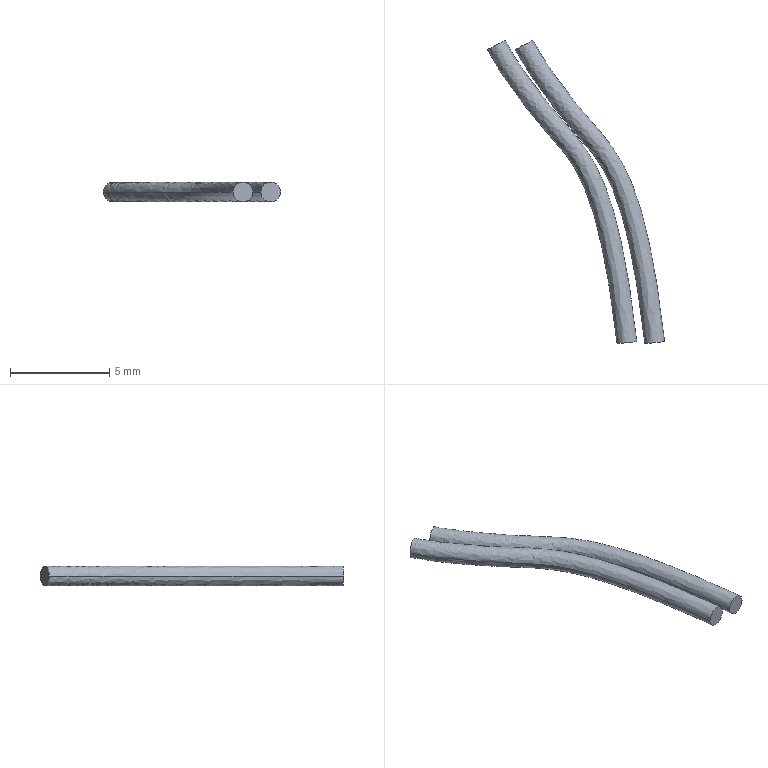Part | SolidWorks | features BaseBody 2 | 2 solids | 8 faces | box 8.921 x 15.285 x 1 mm | volume 26.359 mm3 | plane 4 | spline 4
STEP:
#1=CARTESIAN_POINT('',(-0.4968,-0.05673,0.));
#2=VERTEX_POINT('',#1);
#3=CARTESIAN_POINT('',(0.4968,0.05673,0.));
#4=VERTEX_POINT('',#3);
#5=CARTESIAN_POINT('',(0.,0.,0.));
#6=DIRECTION('',(-0.1135,0.9935,0.));
#7=DIRECTION('',(-0.9935,-0.1135,0.));
#8=AXIS2_PLACEMENT_3D('',#5,#6,#7);
#9=CIRCLE('',#8,0.5);
#10=EDGE_CURVE('',#2,#4,#9,.T.);
#11=ORIENTED_EDGE('',*,*,#10,.F.);
#12=CARTESIAN_POINT('',(0.,0.,0.));
#13=DIRECTION('',(-0.1135,0.9935,0.));
#14=DIRECTION('',(-0.9935,-0.1135,0.));
#15=AXIS2_PLACEMENT_3D('',#12,#13,#14);
#16=CIRCLE('',#15,0.5);
#17=EDGE_CURVE('',#4,#2,#16,.T.);
#18=ORIENTED_EDGE('',*,*,#17,.F.);
#19=EDGE_LOOP('',(#11,#18));
#20=FACE_OUTER_BOUND('',#19,.T.);
#21=CARTESIAN_POINT('',(0.,0.,0.));
#22=DIRECTION('',(-0.1135,0.9935,0.));
#23=DIRECTION('',(0.,0.,1.));
#24=AXIS2_PLACEMENT_3D('',#21,#22,#23);
#25=PLANE('',#24);
#26=ADVANCED_FACE('',(#20),#25,.F.);
#27=CARTESIAN_POINT('',(-7.024,14.772,0.));
#28=VERTEX_POINT('',#27);
#29=CARTESIAN_POINT('',(-6.134,15.228,0.));
#30=VERTEX_POINT('',#29);
#31=CARTESIAN_POINT('',(-6.579,15.,0.));
#32=DIRECTION('',(-0.4556,0.8902,0.));
#33=DIRECTION('',(-0.8902,-0.4556,0.));
#34=AXIS2_PLACEMENT_3D('',#31,#32,#33);
#35=CIRCLE('',#34,0.5);
#36=EDGE_CURVE('',#28,#30,#35,.T.);
#37=ORIENTED_EDGE('',*,*,#36,.T.);
#38=CARTESIAN_POINT('',(-6.579,15.,0.));
#39=DIRECTION('',(-0.4556,0.8902,0.));
#40=DIRECTION('',(-0.8902,-0.4556,0.));
#41=AXIS2_PLACEMENT_3D('',#38,#39,#40);
#42=CIRCLE('',#41,0.5);
#43=EDGE_CURVE('',#30,#28,#42,.T.);
#44=ORIENTED_EDGE('',*,*,#43,.T.);
#45=EDGE_LOOP('',(#37,#44));
#46=FACE_OUTER_BOUND('',#45,.T.);
#47=CARTESIAN_POINT('',(-6.579,15.,0.));
#48=DIRECTION('',(-0.4556,0.8902,0.));
#49=DIRECTION('',(0.,0.,1.));
#50=AXIS2_PLACEMENT_3D('',#47,#48,#49);
#51=PLANE('',#50);
#52=ADVANCED_FACE('',(#46),#51,.T.);
#53=CARTESIAN_POINT('',(0.4968,0.05673,0.));
#54=CARTESIAN_POINT('',(0.03588,4.093,0.));
#55=CARTESIAN_POINT('',(-0.5239,6.452,0.));
#56=CARTESIAN_POINT('',(-1.773,9.573,0.));
#57=CARTESIAN_POINT('',(-2.484,10.33,0.));
#58=CARTESIAN_POINT('',(-4.339,12.439,0.));
#59=CARTESIAN_POINT('',(-5.518,14.024,0.));
#60=CARTESIAN_POINT('',(-6.134,15.228,0.));
#61=B_SPLINE_CURVE_WITH_KNOTS('',3,(#53,#54,#55,#56,#57,#58,#59,#60),.UNSPECIFIED.,.F.,.F.,(4,2,2,4),(0.,0.2491,0.4982,1.),.UNSPECIFIED.);
#62=EDGE_CURVE('',#4,#30,#61,.T.);
#63=ORIENTED_EDGE('',*,*,#62,.F.);
#64=ORIENTED_EDGE('',*,*,#17,.T.);
#65=CARTESIAN_POINT('',(-0.4968,-0.05673,0.));
#66=CARTESIAN_POINT('',(-0.9522,3.932,0.));
#67=CARTESIAN_POINT('',(-1.505,6.213,0.));
#68=CARTESIAN_POINT('',(-2.648,9.069,0.));
#69=CARTESIAN_POINT('',(-3.217,9.649,0.));
#70=CARTESIAN_POINT('',(-5.126,11.82,0.));
#71=CARTESIAN_POINT('',(-6.337,13.429,0.));
#72=CARTESIAN_POINT('',(-7.024,14.772,0.));
#73=B_SPLINE_CURVE_WITH_KNOTS('',3,(#65,#66,#67,#68,#69,#70,#71,#72),.UNSPECIFIED.,.F.,.F.,(4,2,2,4),(0.,0.2491,0.4982,1.),.UNSPECIFIED.);
#74=EDGE_CURVE('',#2,#28,#73,.T.);
#75=ORIENTED_EDGE('',*,*,#74,.T.);
#76=ORIENTED_EDGE('',*,*,#43,.F.);
#77=EDGE_LOOP('',(#63,#64,#75,#76));
#78=FACE_OUTER_BOUND('',#77,.T.);
#79=CARTESIAN_POINT('',(0.4968,0.05673,0.));
#80=CARTESIAN_POINT('',(0.03588,4.093,0.));
#81=CARTESIAN_POINT('',(-0.5239,6.452,0.));
#82=CARTESIAN_POINT('',(-1.773,9.573,0.));
#83=CARTESIAN_POINT('',(-2.484,10.33,0.));
#84=CARTESIAN_POINT('',(-4.339,12.439,0.));
#85=CARTESIAN_POINT('',(-5.518,14.024,0.));
#86=CARTESIAN_POINT('',(-6.134,15.228,0.));
#87=CARTESIAN_POINT('',(0.4968,0.05673,-1.));
#88=CARTESIAN_POINT('',(0.03588,4.093,-1.));
#89=CARTESIAN_POINT('',(-0.5239,6.452,-1.));
#90=CARTESIAN_POINT('',(-1.773,9.573,-1.));
#91=CARTESIAN_POINT('',(-2.484,10.33,-1.));
#92=CARTESIAN_POINT('',(-4.339,12.439,-1.));
#93=CARTESIAN_POINT('',(-5.518,14.024,-1.));
#94=CARTESIAN_POINT('',(-6.134,15.228,-1.));
#95=CARTESIAN_POINT('',(-0.4968,-0.05673,-1.));
#96=CARTESIAN_POINT('',(-0.9522,3.932,-1.));
#97=CARTESIAN_POINT('',(-1.505,6.213,-1.));
#98=CARTESIAN_POINT('',(-2.648,9.069,-1.));
#99=CARTESIAN_POINT('',(-3.217,9.649,-1.));
#100=CARTESIAN_POINT('',(-5.126,11.82,-1.));
#101=CARTESIAN_POINT('',(-6.337,13.429,-1.));
#102=CARTESIAN_POINT('',(-7.024,14.772,-1.));
#103=CARTESIAN_POINT('',(-0.4968,-0.05673,0.));
#104=CARTESIAN_POINT('',(-0.9522,3.932,0.));
#105=CARTESIAN_POINT('',(-1.505,6.213,0.));
#106=CARTESIAN_POINT('',(-2.648,9.069,0.));
#107=CARTESIAN_POINT('',(-3.217,9.649,0.));
#108=CARTESIAN_POINT('',(-5.126,11.82,0.));
#109=CARTESIAN_POINT('',(-6.337,13.429,0.));
#110=CARTESIAN_POINT('',(-7.024,14.772,0.));
#111=(BOUNDED_SURFACE()B_SPLINE_SURFACE(3,3,((#79,#80,#81,#82,#83,#84,#85,#86),(#87,#88,#89,#90,#91,#92,#93,#94),(#95,#96,#97,#98,#99,#100,#101,#102),(#103,#104,#105,#106,#107,#108,#109,#110)),.UNSPECIFIED.,.F.,.F.,.F.)B_SPLINE_SURFACE_WITH_KNOTS((4,4),(4,2,2,4),(0.5,1.),(0.,0.2491,0.4982,1.),.UNSPECIFIED.)GEOMETRIC_REPRESENTATION_ITEM()RATIONAL_B_SPLINE_SURFACE(((1.,1.,1.,1.,1.,1.,1.,1.),(0.3333,0.3333,0.3333,0.3333,0.3333,0.3333,0.3333,0.3333),(0.3333,0.3333,0.3333,0.3333,0.3333,0.3333,0.3333,0.3333),(1.,1.,1.,1.,1.,1.,1.,1.)))REPRESENTATION_ITEM('')SURFACE());
#112=ADVANCED_FACE('',(#78),#111,.T.);
#113=ORIENTED_EDGE('',*,*,#10,.T.);
#114=ORIENTED_EDGE('',*,*,#62,.T.);
#115=ORIENTED_EDGE('',*,*,#36,.F.);
#116=ORIENTED_EDGE('',*,*,#74,.F.);
#117=EDGE_LOOP('',(#113,#114,#115,#116));
#118=FACE_OUTER_BOUND('',#117,.T.);
#119=CARTESIAN_POINT('',(-0.4968,-0.05673,0.));
#120=CARTESIAN_POINT('',(-0.9522,3.932,0.));
#121=CARTESIAN_POINT('',(-1.505,6.213,0.));
#122=CARTESIAN_POINT('',(-2.648,9.069,0.));
#123=CARTESIAN_POINT('',(-3.217,9.649,0.));
#124=CARTESIAN_POINT('',(-5.126,11.82,0.));
#125=CARTESIAN_POINT('',(-6.337,13.429,0.));
#126=CARTESIAN_POINT('',(-7.024,14.772,0.));
#127=CARTESIAN_POINT('',(-0.4968,-0.05673,1.));
#128=CARTESIAN_POINT('',(-0.9522,3.932,1.));
#129=CARTESIAN_POINT('',(-1.505,6.213,1.));
#130=CARTESIAN_POINT('',(-2.648,9.069,1.));
#131=CARTESIAN_POINT('',(-3.217,9.649,1.));
#132=CARTESIAN_POINT('',(-5.126,11.82,1.));
#133=CARTESIAN_POINT('',(-6.337,13.429,1.));
#134=CARTESIAN_POINT('',(-7.024,14.772,1.));
#135=CARTESIAN_POINT('',(0.4968,0.05673,1.));
#136=CARTESIAN_POINT('',(0.03588,4.093,1.));
#137=CARTESIAN_POINT('',(-0.5239,6.452,1.));
#138=CARTESIAN_POINT('',(-1.773,9.573,1.));
#139=CARTESIAN_POINT('',(-2.484,10.33,1.));
#140=CARTESIAN_POINT('',(-4.339,12.439,1.));
#141=CARTESIAN_POINT('',(-5.518,14.024,1.));
#142=CARTESIAN_POINT('',(-6.134,15.228,1.));
#143=CARTESIAN_POINT('',(0.4968,0.05673,0.));
#144=CARTESIAN_POINT('',(0.03588,4.093,0.));
#145=CARTESIAN_POINT('',(-0.5239,6.452,0.));
#146=CARTESIAN_POINT('',(-1.773,9.573,0.));
#147=CARTESIAN_POINT('',(-2.484,10.33,0.));
#148=CARTESIAN_POINT('',(-4.339,12.439,0.));
#149=CARTESIAN_POINT('',(-5.518,14.024,0.));
#150=CARTESIAN_POINT('',(-6.134,15.228,0.));
#151=(BOUNDED_SURFACE()B_SPLINE_SURFACE(3,3,((#119,#120,#121,#122,#123,#124,#125,#126),(#127,#128,#129,#130,#131,#132,#133,#134),(#135,#136,#137,#138,#139,#140,#141,#142),(#143,#144,#145,#146,#147,#148,#149,#150)),.UNSPECIFIED.,.F.,.F.,.F.)B_SPLINE_SURFACE_WITH_KNOTS((4,4),(4,2,2,4),(0.,0.5),(0.,0.2491,0.4982,1.),.UNSPECIFIED.)GEOMETRIC_REPRESENTATION_ITEM()RATIONAL_B_SPLINE_SURFACE(((1.,1.,1.,1.,1.,1.,1.,1.),(0.3333,0.3333,0.3333,0.3333,0.3333,0.3333,0.3333,0.3333),(0.3333,0.3333,0.3333,0.3333,0.3333,0.3333,0.3333,0.3333),(1.,1.,1.,1.,1.,1.,1.,1.)))REPRESENTATION_ITEM('')SURFACE());
#152=ADVANCED_FACE('',(#118),#151,.T.);
#153=CLOSED_SHELL('',(#26,#52,#112,#152));
#154=MANIFOLD_SOLID_BREP('',#153);
#155=CARTESIAN_POINT('',(0.9032,-0.05673,0.));
#156=VERTEX_POINT('',#155);
#157=CARTESIAN_POINT('',(1.897,0.05673,0.));
#158=VERTEX_POINT('',#157);
#159=CARTESIAN_POINT('',(1.4,0.,0.));
#160=DIRECTION('',(-0.1135,0.9935,0.));
#161=DIRECTION('',(-0.9935,-0.1135,0.));
#162=AXIS2_PLACEMENT_3D('',#159,#160,#161);
#163=CIRCLE('',#162,0.5);
#164=EDGE_CURVE('',#156,#158,#163,.T.);
#165=ORIENTED_EDGE('',*,*,#164,.F.);
#166=CARTESIAN_POINT('',(1.4,0.,0.));
#167=DIRECTION('',(-0.1135,0.9935,0.));
#168=DIRECTION('',(-0.9935,-0.1135,0.));
#169=AXIS2_PLACEMENT_3D('',#166,#167,#168);
#170=CIRCLE('',#169,0.5);
#171=EDGE_CURVE('',#158,#156,#170,.T.);
#172=ORIENTED_EDGE('',*,*,#171,.F.);
#173=EDGE_LOOP('',(#165,#172));
#174=FACE_OUTER_BOUND('',#173,.T.);
#175=CARTESIAN_POINT('',(1.4,0.,0.));
#176=DIRECTION('',(-0.1135,0.9935,0.));
#177=DIRECTION('',(0.,0.,1.));
#178=AXIS2_PLACEMENT_3D('',#175,#176,#177);
#179=PLANE('',#178);
#180=ADVANCED_FACE('',(#174),#179,.F.);
#181=CARTESIAN_POINT('',(-5.624,14.772,0.));
#182=VERTEX_POINT('',#181);
#183=CARTESIAN_POINT('',(-4.734,15.228,0.));
#184=VERTEX_POINT('',#183);
#185=CARTESIAN_POINT('',(-5.179,15.,0.));
#186=DIRECTION('',(-0.4556,0.8902,0.));
#187=DIRECTION('',(-0.8902,-0.4556,0.));
#188=AXIS2_PLACEMENT_3D('',#185,#186,#187);
#189=CIRCLE('',#188,0.5);
#190=EDGE_CURVE('',#182,#184,#189,.T.);
#191=ORIENTED_EDGE('',*,*,#190,.T.);
#192=CARTESIAN_POINT('',(-5.179,15.,0.));
#193=DIRECTION('',(-0.4556,0.8902,0.));
#194=DIRECTION('',(-0.8902,-0.4556,0.));
#195=AXIS2_PLACEMENT_3D('',#192,#193,#194);
#196=CIRCLE('',#195,0.5);
#197=EDGE_CURVE('',#184,#182,#196,.T.);
#198=ORIENTED_EDGE('',*,*,#197,.T.);
#199=EDGE_LOOP('',(#191,#198));
#200=FACE_OUTER_BOUND('',#199,.T.);
#201=CARTESIAN_POINT('',(-5.179,15.,0.));
#202=DIRECTION('',(-0.4556,0.8902,0.));
#203=DIRECTION('',(0.,0.,1.));
#204=AXIS2_PLACEMENT_3D('',#201,#202,#203);
#205=PLANE('',#204);
#206=ADVANCED_FACE('',(#200),#205,.T.);
#207=CARTESIAN_POINT('',(1.897,0.05673,0.));
#208=CARTESIAN_POINT('',(1.436,4.093,0.));
#209=CARTESIAN_POINT('',(0.8761,6.452,0.));
#210=CARTESIAN_POINT('',(-0.3732,9.573,0.));
#211=CARTESIAN_POINT('',(-1.084,10.33,0.));
#212=CARTESIAN_POINT('',(-2.939,12.439,0.));
#213=CARTESIAN_POINT('',(-4.118,14.024,0.));
#214=CARTESIAN_POINT('',(-4.734,15.228,0.));
#215=B_SPLINE_CURVE_WITH_KNOTS('',3,(#207,#208,#209,#210,#211,#212,#213,#214),.UNSPECIFIED.,.F.,.F.,(4,2,2,4),(0.,0.2491,0.4982,1.),.UNSPECIFIED.);
#216=EDGE_CURVE('',#158,#184,#215,.T.);
#217=ORIENTED_EDGE('',*,*,#216,.F.);
#218=ORIENTED_EDGE('',*,*,#171,.T.);
#219=CARTESIAN_POINT('',(0.9032,-0.05673,0.));
#220=CARTESIAN_POINT('',(0.4478,3.932,0.));
#221=CARTESIAN_POINT('',(-0.1055,6.213,0.));
#222=CARTESIAN_POINT('',(-1.248,9.069,0.));
#223=CARTESIAN_POINT('',(-1.817,9.649,0.));
#224=CARTESIAN_POINT('',(-3.726,11.82,0.));
#225=CARTESIAN_POINT('',(-4.937,13.429,0.));
#226=CARTESIAN_POINT('',(-5.624,14.772,0.));
#227=B_SPLINE_CURVE_WITH_KNOTS('',3,(#219,#220,#221,#222,#223,#224,#225,#226),.UNSPECIFIED.,.F.,.F.,(4,2,2,4),(0.,0.2491,0.4982,1.),.UNSPECIFIED.);
#228=EDGE_CURVE('',#156,#182,#227,.T.);
#229=ORIENTED_EDGE('',*,*,#228,.T.);
#230=ORIENTED_EDGE('',*,*,#197,.F.);
#231=EDGE_LOOP('',(#217,#218,#229,#230));
#232=FACE_OUTER_BOUND('',#231,.T.);
#233=CARTESIAN_POINT('',(1.897,0.05673,0.));
#234=CARTESIAN_POINT('',(1.436,4.093,0.));
#235=CARTESIAN_POINT('',(0.8761,6.452,0.));
#236=CARTESIAN_POINT('',(-0.3732,9.573,0.));
#237=CARTESIAN_POINT('',(-1.084,10.33,0.));
#238=CARTESIAN_POINT('',(-2.939,12.439,0.));
#239=CARTESIAN_POINT('',(-4.118,14.024,0.));
#240=CARTESIAN_POINT('',(-4.734,15.228,0.));
#241=CARTESIAN_POINT('',(1.897,0.05673,-1.));
#242=CARTESIAN_POINT('',(1.436,4.093,-1.));
#243=CARTESIAN_POINT('',(0.8761,6.452,-1.));
#244=CARTESIAN_POINT('',(-0.3732,9.573,-1.));
#245=CARTESIAN_POINT('',(-1.084,10.33,-1.));
#246=CARTESIAN_POINT('',(-2.939,12.439,-1.));
#247=CARTESIAN_POINT('',(-4.118,14.024,-1.));
#248=CARTESIAN_POINT('',(-4.734,15.228,-1.));
#249=CARTESIAN_POINT('',(0.9032,-0.05673,-1.));
#250=CARTESIAN_POINT('',(0.4478,3.932,-1.));
#251=CARTESIAN_POINT('',(-0.1055,6.213,-1.));
#252=CARTESIAN_POINT('',(-1.248,9.069,-1.));
#253=CARTESIAN_POINT('',(-1.817,9.649,-1.));
#254=CARTESIAN_POINT('',(-3.726,11.82,-1.));
#255=CARTESIAN_POINT('',(-4.937,13.429,-1.));
#256=CARTESIAN_POINT('',(-5.624,14.772,-1.));
#257=CARTESIAN_POINT('',(0.9032,-0.05673,0.));
#258=CARTESIAN_POINT('',(0.4478,3.932,0.));
#259=CARTESIAN_POINT('',(-0.1055,6.213,0.));
#260=CARTESIAN_POINT('',(-1.248,9.069,0.));
#261=CARTESIAN_POINT('',(-1.817,9.649,0.));
#262=CARTESIAN_POINT('',(-3.726,11.82,0.));
#263=CARTESIAN_POINT('',(-4.937,13.429,0.));
#264=CARTESIAN_POINT('',(-5.624,14.772,0.));
#265=(BOUNDED_SURFACE()B_SPLINE_SURFACE(3,3,((#233,#234,#235,#236,#237,#238,#239,#240),(#241,#242,#243,#244,#245,#246,#247,#248),(#249,#250,#251,#252,#253,#254,#255,#256),(#257,#258,#259,#260,#261,#262,#263,#264)),.UNSPECIFIED.,.F.,.F.,.T.)B_SPLINE_SURFACE_WITH_KNOTS((4,4),(4,2,2,4),(0.5,1.),(0.,0.2491,0.4982,1.),.UNSPECIFIED.)GEOMETRIC_REPRESENTATION_ITEM()RATIONAL_B_SPLINE_SURFACE(((1.,1.,1.,1.,1.,1.,1.,1.),(0.3333,0.3333,0.3333,0.3333,0.3333,0.3333,0.3333,0.3333),(0.3333,0.3333,0.3333,0.3333,0.3333,0.3333,0.3333,0.3333),(1.,1.,1.,1.,1.,1.,1.,1.)))REPRESENTATION_ITEM('')SURFACE());
#266=ADVANCED_FACE('',(#232),#265,.T.);
#267=ORIENTED_EDGE('',*,*,#164,.T.);
#268=ORIENTED_EDGE('',*,*,#216,.T.);
#269=ORIENTED_EDGE('',*,*,#190,.F.);
#270=ORIENTED_EDGE('',*,*,#228,.F.);
#271=EDGE_LOOP('',(#267,#268,#269,#270));
#272=FACE_OUTER_BOUND('',#271,.T.);
#273=CARTESIAN_POINT('',(0.9032,-0.05673,0.));
#274=CARTESIAN_POINT('',(0.4478,3.932,0.));
#275=CARTESIAN_POINT('',(-0.1055,6.213,0.));
#276=CARTESIAN_POINT('',(-1.248,9.069,0.));
#277=CARTESIAN_POINT('',(-1.817,9.649,0.));
#278=CARTESIAN_POINT('',(-3.726,11.82,0.));
#279=CARTESIAN_POINT('',(-4.937,13.429,0.));
#280=CARTESIAN_POINT('',(-5.624,14.772,0.));
#281=CARTESIAN_POINT('',(0.9032,-0.05673,1.));
#282=CARTESIAN_POINT('',(0.4478,3.932,1.));
#283=CARTESIAN_POINT('',(-0.1055,6.213,1.));
#284=CARTESIAN_POINT('',(-1.248,9.069,1.));
#285=CARTESIAN_POINT('',(-1.817,9.649,1.));
#286=CARTESIAN_POINT('',(-3.726,11.82,1.));
#287=CARTESIAN_POINT('',(-4.937,13.429,1.));
#288=CARTESIAN_POINT('',(-5.624,14.772,1.));
#289=CARTESIAN_POINT('',(1.897,0.05673,1.));
#290=CARTESIAN_POINT('',(1.436,4.093,1.));
#291=CARTESIAN_POINT('',(0.8761,6.452,1.));
#292=CARTESIAN_POINT('',(-0.3732,9.573,1.));
#293=CARTESIAN_POINT('',(-1.084,10.33,1.));
#294=CARTESIAN_POINT('',(-2.939,12.439,1.));
#295=CARTESIAN_POINT('',(-4.118,14.024,1.));
#296=CARTESIAN_POINT('',(-4.734,15.228,1.));
#297=CARTESIAN_POINT('',(1.897,0.05673,0.));
#298=CARTESIAN_POINT('',(1.436,4.093,0.));
#299=CARTESIAN_POINT('',(0.8761,6.452,0.));
#300=CARTESIAN_POINT('',(-0.3732,9.573,0.));
#301=CARTESIAN_POINT('',(-1.084,10.33,0.));
#302=CARTESIAN_POINT('',(-2.939,12.439,0.));
#303=CARTESIAN_POINT('',(-4.118,14.024,0.));
#304=CARTESIAN_POINT('',(-4.734,15.228,0.));
#305=(BOUNDED_SURFACE()B_SPLINE_SURFACE(3,3,((#273,#274,#275,#276,#277,#278,#279,#280),(#281,#282,#283,#284,#285,#286,#287,#288),(#289,#290,#291,#292,#293,#294,#295,#296),(#297,#298,#299,#300,#301,#302,#303,#304)),.UNSPECIFIED.,.F.,.F.,.F.)B_SPLINE_SURFACE_WITH_KNOTS((4,4),(4,2,2,4),(0.,0.5),(0.,0.2491,0.4982,1.),.UNSPECIFIED.)GEOMETRIC_REPRESENTATION_ITEM()RATIONAL_B_SPLINE_SURFACE(((1.,1.,1.,1.,1.,1.,1.,1.),(0.3333,0.3333,0.3333,0.3333,0.3333,0.3333,0.3333,0.3333),(0.3333,0.3333,0.3333,0.3333,0.3333,0.3333,0.3333,0.3333),(1.,1.,1.,1.,1.,1.,1.,1.)))REPRESENTATION_ITEM('')SURFACE());
#306=ADVANCED_FACE('',(#272),#305,.T.);
#307=CLOSED_SHELL('',(#180,#206,#266,#306));
#308=MANIFOLD_SOLID_BREP('',#307);
#309=CARTESIAN_POINT('',(0.,0.,0.));
#310=DIRECTION('',(0.,0.,1.));
#311=DIRECTION('',(1.,0.,0.));
#312=AXIS2_PLACEMENT_3D('',#309,#310,#311);
#313=(LENGTH_UNIT()NAMED_UNIT(*)SI_UNIT(.MILLI.,.METRE.));
#314=UNCERTAINTY_MEASURE_WITH_UNIT(LENGTH_MEASURE(0.00001),#313,'','');
#315=(NAMED_UNIT(*)PLANE_ANGLE_UNIT()SI_UNIT($,.RADIAN.));
#316=(NAMED_UNIT(*)SI_UNIT($,.STERADIAN.)SOLID_ANGLE_UNIT());
#317=(GEOMETRIC_REPRESENTATION_CONTEXT(3)GLOBAL_UNCERTAINTY_ASSIGNED_CONTEXT((#314))GLOBAL_UNIT_ASSIGNED_CONTEXT((#313,#315,#316))REPRESENTATION_CONTEXT('',''));
#318=ADVANCED_BREP_SHAPE_REPRESENTATION('',(#154,#308,#312),#317);